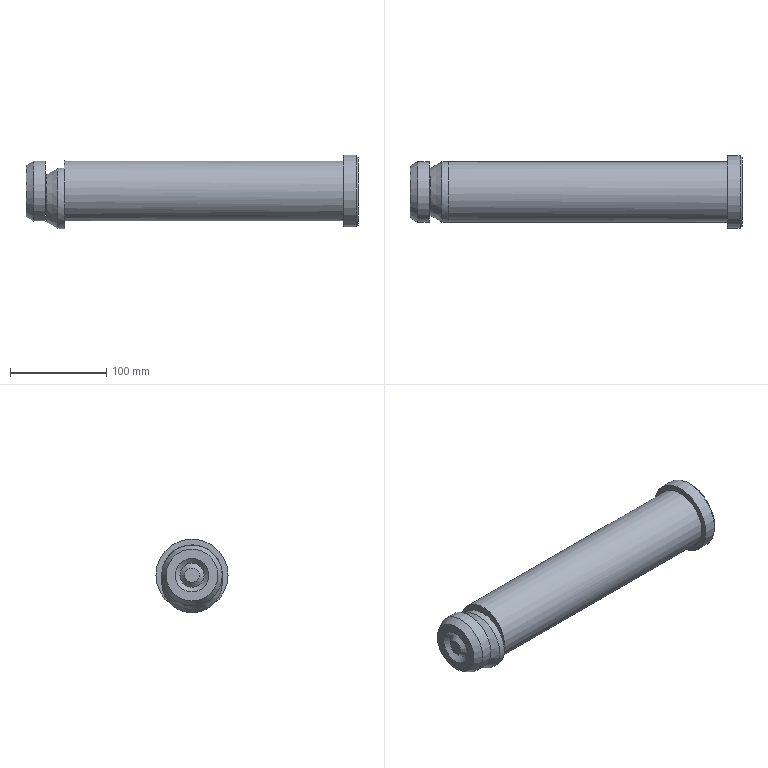Part | NX | features MAIN_BODY 2 | 1 solid | 24 faces | box 345 x 75 x 76.5 mm | volume 1062579 mm3 | plane 10 | cylinder 8 | cone 6 | commonest cylinder face diameters 63 x3 25 x1 25.1 x1 30 x1 44.6 x1 75 x1
STEP:
#1=CARTESIAN_POINT('',(1229.,875.809,-265.597));
#2=VERTEX_POINT('',#1);
#3=CARTESIAN_POINT('',(1229.,884.191,-265.597));
#4=VERTEX_POINT('',#3);
#5=CARTESIAN_POINT('',(1229.,880.,-287.5));
#6=DIRECTION('',(1.,0.,0.));
#7=DIRECTION('',(0.,1.,0.));
#8=AXIS2_PLACEMENT_3D('',#5,#6,#7);
#9=CIRCLE('',#8,22.3);
#10=EDGE_CURVE('',#2,#4,#9,.T.);
#11=ORIENTED_EDGE('',*,*,#10,.F.);
#12=CARTESIAN_POINT('',(1229.,880.,-280.));
#13=DIRECTION('',(1.,0.,0.));
#14=DIRECTION('',(0.,1.,0.));
#15=AXIS2_PLACEMENT_3D('',#12,#13,#14);
#16=CIRCLE('',#15,15.);
#17=EDGE_CURVE('',#2,#4,#16,.T.);
#18=ORIENTED_EDGE('',*,*,#17,.T.);
#19=EDGE_LOOP('',(#11,#18));
#20=FACE_BOUND('',#19,.T.);
#21=CARTESIAN_POINT('',(1229.,880.,-280.));
#22=DIRECTION('',(1.,0.,0.));
#23=DIRECTION('',(0.,1.,0.));
#24=AXIS2_PLACEMENT_3D('',#21,#22,#23);
#25=PLANE('',#24);
#26=ADVANCED_FACE('',(#20),#25,.F.);
#27=CARTESIAN_POINT('',(1209.,895.,-280.));
#28=VERTEX_POINT('',#27);
#29=CARTESIAN_POINT('',(1209.,880.,-280.));
#30=DIRECTION('',(1.,0.,0.));
#31=DIRECTION('',(0.,1.,0.));
#32=AXIS2_PLACEMENT_3D('',#29,#30,#31);
#33=CIRCLE('',#32,15.);
#34=EDGE_CURVE('',#28,#28,#33,.F.);
#35=ORIENTED_EDGE('',*,*,#34,.F.);
#36=EDGE_LOOP('',(#35));
#37=FACE_BOUND('',#36,.T.);
#38=CARTESIAN_POINT('',(1210.,875.809,-265.597));
#39=VERTEX_POINT('',#38);
#40=CARTESIAN_POINT('',(1210.,884.191,-265.597));
#41=VERTEX_POINT('',#40);
#42=CARTESIAN_POINT('',(1210.,880.,-280.));
#43=DIRECTION('',(1.,0.,0.));
#44=DIRECTION('',(0.,1.,0.));
#45=AXIS2_PLACEMENT_3D('',#42,#43,#44);
#46=CIRCLE('',#45,15.);
#47=EDGE_CURVE('',#39,#41,#46,.F.);
#48=ORIENTED_EDGE('',*,*,#47,.T.);
#49=CARTESIAN_POINT('',(1219.6,884.191,-265.597));
#50=DIRECTION('',(1.,0.,0.));
#51=VECTOR('',#50,1000.);
#52=LINE('',#49,#51);
#53=EDGE_CURVE('',#41,#4,#52,.T.);
#54=ORIENTED_EDGE('',*,*,#53,.T.);
#55=ORIENTED_EDGE('',*,*,#17,.F.);
#56=CARTESIAN_POINT('',(1219.6,875.809,-265.597));
#57=DIRECTION('',(1.,0.,0.));
#58=VECTOR('',#57,1000.);
#59=LINE('',#56,#58);
#60=EDGE_CURVE('',#2,#39,#59,.F.);
#61=ORIENTED_EDGE('',*,*,#60,.T.);
#62=EDGE_LOOP('',(#48,#54,#55,#61));
#63=FACE_BOUND('',#62,.T.);
#64=CARTESIAN_POINT('',(1209.,880.,-280.));
#65=DIRECTION('',(1.,0.,0.));
#66=DIRECTION('',(0.,1.,0.));
#67=AXIS2_PLACEMENT_3D('',#64,#65,#66);
#68=CYLINDRICAL_SURFACE('',#67,15.);
#69=ADVANCED_FACE('',(#37,#63),#68,.T.);
#70=CARTESIAN_POINT('',(1208.2,892.55,-280.));
#71=VERTEX_POINT('',#70);
#72=CARTESIAN_POINT('',(1208.2,880.,-280.));
#73=DIRECTION('',(1.,0.,0.));
#74=DIRECTION('',(0.,1.,0.));
#75=AXIS2_PLACEMENT_3D('',#72,#73,#74);
#76=CIRCLE('',#75,12.55);
#77=EDGE_CURVE('',#71,#71,#76,.T.);
#78=ORIENTED_EDGE('',*,*,#77,.T.);
#79=EDGE_LOOP('',(#78));
#80=FACE_BOUND('',#79,.T.);
#81=CARTESIAN_POINT('',(1194.,892.55,-280.));
#82=VERTEX_POINT('',#81);
#83=CARTESIAN_POINT('',(1194.,880.,-280.));
#84=DIRECTION('',(1.,0.,0.));
#85=DIRECTION('',(0.,1.,0.));
#86=AXIS2_PLACEMENT_3D('',#83,#84,#85);
#87=CIRCLE('',#86,12.55);
#88=EDGE_CURVE('',#82,#82,#87,.F.);
#89=ORIENTED_EDGE('',*,*,#88,.T.);
#90=EDGE_LOOP('',(#89));
#91=FACE_BOUND('',#90,.T.);
#92=CARTESIAN_POINT('',(1189.,880.,-280.));
#93=DIRECTION('',(1.,0.,0.));
#94=DIRECTION('',(0.,1.,0.));
#95=AXIS2_PLACEMENT_3D('',#92,#93,#94);
#96=CYLINDRICAL_SURFACE('',#95,12.55);
#97=ADVANCED_FACE('',(#80,#91),#96,.F.);
#98=CARTESIAN_POINT('',(1197.,911.5,-280.));
#99=VERTEX_POINT('',#98);
#100=CARTESIAN_POINT('',(1197.,880.,-280.));
#101=DIRECTION('',(1.,0.,0.));
#102=DIRECTION('',(0.,1.,0.));
#103=AXIS2_PLACEMENT_3D('',#100,#101,#102);
#104=CIRCLE('',#103,31.5);
#105=EDGE_CURVE('',#99,#99,#104,.T.);
#106=ORIENTED_EDGE('',*,*,#105,.T.);
#107=EDGE_LOOP('',(#106));
#108=FACE_BOUND('',#107,.T.);
#109=CARTESIAN_POINT('',(1209.,911.5,-280.));
#110=VERTEX_POINT('',#109);
#111=CARTESIAN_POINT('',(1209.,880.,-280.));
#112=DIRECTION('',(1.,0.,0.));
#113=DIRECTION('',(0.,1.,0.));
#114=AXIS2_PLACEMENT_3D('',#111,#112,#113);
#115=CIRCLE('',#114,31.5);
#116=EDGE_CURVE('',#110,#110,#115,.T.);
#117=ORIENTED_EDGE('',*,*,#116,.F.);
#118=EDGE_LOOP('',(#117));
#119=FACE_BOUND('',#118,.T.);
#120=CARTESIAN_POINT('',(1189.,880.,-280.));
#121=DIRECTION('',(1.,0.,0.));
#122=DIRECTION('',(0.,1.,0.));
#123=AXIS2_PLACEMENT_3D('',#120,#121,#122);
#124=CYLINDRICAL_SURFACE('',#123,31.5);
#125=ADVANCED_FACE('',(#108,#119),#124,.T.);
#126=CARTESIAN_POINT('',(1189.,897.55,-280.));
#127=VERTEX_POINT('',#126);
#128=CARTESIAN_POINT('',(1189.,880.,-280.));
#129=DIRECTION('',(1.,0.,0.));
#130=DIRECTION('',(0.,1.,0.));
#131=AXIS2_PLACEMENT_3D('',#128,#129,#130);
#132=CIRCLE('',#131,17.55);
#133=EDGE_CURVE('',#127,#127,#132,.T.);
#134=ORIENTED_EDGE('',*,*,#133,.T.);
#135=EDGE_LOOP('',(#134));
#136=FACE_BOUND('',#135,.T.);
#137=CARTESIAN_POINT('',(1189.,906.881,-280.));
#138=VERTEX_POINT('',#137);
#139=CARTESIAN_POINT('',(1189.,880.,-280.));
#140=DIRECTION('',(1.,0.,0.));
#141=DIRECTION('',(0.,1.,0.));
#142=AXIS2_PLACEMENT_3D('',#139,#140,#141);
#143=CIRCLE('',#142,26.881);
#144=EDGE_CURVE('',#138,#138,#143,.F.);
#145=ORIENTED_EDGE('',*,*,#144,.T.);
#146=EDGE_LOOP('',(#145));
#147=FACE_BOUND('',#146,.T.);
#148=CARTESIAN_POINT('',(1189.,880.,-280.));
#149=DIRECTION('',(1.,0.,0.));
#150=DIRECTION('',(0.,1.,0.));
#151=AXIS2_PLACEMENT_3D('',#148,#149,#150);
#152=PLANE('',#151);
#153=ADVANCED_FACE('',(#136,#147),#152,.F.);
#154=ORIENTED_EDGE('',*,*,#34,.T.);
#155=EDGE_LOOP('',(#154));
#156=FACE_BOUND('',#155,.T.);
#157=ORIENTED_EDGE('',*,*,#116,.T.);
#158=EDGE_LOOP('',(#157));
#159=FACE_BOUND('',#158,.T.);
#160=CARTESIAN_POINT('',(1209.,880.,-280.));
#161=DIRECTION('',(1.,0.,0.));
#162=DIRECTION('',(0.,1.,0.));
#163=AXIS2_PLACEMENT_3D('',#160,#161,#162);
#164=PLANE('',#163);
#165=ADVANCED_FACE('',(#156,#159),#164,.T.);
#166=ORIENTED_EDGE('',*,*,#144,.F.);
#167=EDGE_LOOP('',(#166));
#168=FACE_BOUND('',#167,.T.);
#169=ORIENTED_EDGE('',*,*,#105,.F.);
#170=EDGE_LOOP('',(#169));
#171=FACE_BOUND('',#170,.T.);
#172=CARTESIAN_POINT('',(1197.,880.,-280.));
#173=DIRECTION('',(1.,0.,0.));
#174=DIRECTION('',(0.,1.,0.));
#175=AXIS2_PLACEMENT_3D('',#172,#173,#174);
#176=CONICAL_SURFACE('',#175,31.5,0.5236);
#177=ADVANCED_FACE('',(#168,#171),#176,.T.);
#178=ORIENTED_EDGE('',*,*,#88,.F.);
#179=EDGE_LOOP('',(#178));
#180=FACE_BOUND('',#179,.T.);
#181=ORIENTED_EDGE('',*,*,#133,.F.);
#182=EDGE_LOOP('',(#181));
#183=FACE_BOUND('',#182,.T.);
#184=CARTESIAN_POINT('',(1189.,880.,-280.));
#185=DIRECTION('',(-1.,0.,0.));
#186=DIRECTION('',(0.,-1.,0.));
#187=AXIS2_PLACEMENT_3D('',#184,#185,#186);
#188=CONICAL_SURFACE('',#187,17.55,0.7854);
#189=ADVANCED_FACE('',(#180,#183),#188,.F.);
#190=CARTESIAN_POINT('',(1209.,893.35,-280.));
#191=VERTEX_POINT('',#190);
#192=CARTESIAN_POINT('',(1209.,880.,-280.));
#193=DIRECTION('',(1.,0.,0.));
#194=DIRECTION('',(0.,1.,0.));
#195=AXIS2_PLACEMENT_3D('',#192,#193,#194);
#196=CIRCLE('',#195,13.35);
#197=EDGE_CURVE('',#191,#191,#196,.F.);
#198=ORIENTED_EDGE('',*,*,#197,.F.);
#199=EDGE_LOOP('',(#198));
#200=FACE_BOUND('',#199,.T.);
#201=ORIENTED_EDGE('',*,*,#77,.F.);
#202=EDGE_LOOP('',(#201));
#203=FACE_BOUND('',#202,.T.);
#204=CARTESIAN_POINT('',(1208.2,880.,-280.));
#205=DIRECTION('',(1.,0.,0.));
#206=DIRECTION('',(0.,1.,0.));
#207=AXIS2_PLACEMENT_3D('',#204,#205,#206);
#208=CONICAL_SURFACE('',#207,12.55,0.7854);
#209=ADVANCED_FACE('',(#200,#203),#208,.F.);
#210=CARTESIAN_POINT('',(1189.,887.5,-280.));
#211=VERTEX_POINT('',#210);
#212=CARTESIAN_POINT('',(1189.,880.,-280.));
#213=DIRECTION('',(1.,0.,0.));
#214=DIRECTION('',(0.,1.,0.));
#215=AXIS2_PLACEMENT_3D('',#212,#213,#214);
#216=CIRCLE('',#215,7.5);
#217=EDGE_CURVE('',#211,#211,#216,.F.);
#218=ORIENTED_EDGE('',*,*,#217,.T.);
#219=EDGE_LOOP('',(#218));
#220=FACE_BOUND('',#219,.T.);
#221=CARTESIAN_POINT('',(1189.,880.,-280.));
#222=DIRECTION('',(1.,0.,0.));
#223=DIRECTION('',(0.,1.,0.));
#224=AXIS2_PLACEMENT_3D('',#221,#222,#223);
#225=PLANE('',#224);
#226=ADVANCED_FACE('',(#220),#225,.F.);
#227=ORIENTED_EDGE('',*,*,#217,.F.);
#228=EDGE_LOOP('',(#227));
#229=FACE_BOUND('',#228,.T.);
#230=CARTESIAN_POINT('',(1194.,892.5,-280.));
#231=VERTEX_POINT('',#230);
#232=CARTESIAN_POINT('',(1194.,880.,-280.));
#233=DIRECTION('',(1.,0.,0.));
#234=DIRECTION('',(0.,1.,0.));
#235=AXIS2_PLACEMENT_3D('',#232,#233,#234);
#236=CIRCLE('',#235,12.5);
#237=EDGE_CURVE('',#231,#231,#236,.T.);
#238=ORIENTED_EDGE('',*,*,#237,.F.);
#239=EDGE_LOOP('',(#238));
#240=FACE_BOUND('',#239,.T.);
#241=CARTESIAN_POINT('',(1194.,880.,-280.));
#242=DIRECTION('',(1.,0.,0.));
#243=DIRECTION('',(0.,1.,0.));
#244=AXIS2_PLACEMENT_3D('',#241,#242,#243);
#245=CONICAL_SURFACE('',#244,12.5,0.7854);
#246=ADVANCED_FACE('',(#229,#240),#245,.T.);
#247=ORIENTED_EDGE('',*,*,#237,.T.);
#248=EDGE_LOOP('',(#247));
#249=FACE_BOUND('',#248,.T.);
#250=CARTESIAN_POINT('',(1209.,892.5,-280.));
#251=VERTEX_POINT('',#250);
#252=CARTESIAN_POINT('',(1209.,880.,-280.));
#253=DIRECTION('',(1.,0.,0.));
#254=DIRECTION('',(0.,1.,0.));
#255=AXIS2_PLACEMENT_3D('',#252,#253,#254);
#256=CIRCLE('',#255,12.5);
#257=EDGE_CURVE('',#251,#251,#256,.T.);
#258=ORIENTED_EDGE('',*,*,#257,.F.);
#259=EDGE_LOOP('',(#258));
#260=FACE_BOUND('',#259,.T.);
#261=CARTESIAN_POINT('',(1189.,880.,-280.));
#262=DIRECTION('',(1.,0.,0.));
#263=DIRECTION('',(0.,1.,0.));
#264=AXIS2_PLACEMENT_3D('',#261,#262,#263);
#265=CYLINDRICAL_SURFACE('',#264,12.5);
#266=ADVANCED_FACE('',(#249,#260),#265,.T.);
#267=ORIENTED_EDGE('',*,*,#197,.T.);
#268=EDGE_LOOP('',(#267));
#269=FACE_BOUND('',#268,.T.);
#270=ORIENTED_EDGE('',*,*,#257,.T.);
#271=EDGE_LOOP('',(#270));
#272=FACE_BOUND('',#271,.T.);
#273=CARTESIAN_POINT('',(1209.,880.,-280.));
#274=DIRECTION('',(1.,0.,0.));
#275=DIRECTION('',(0.,1.,0.));
#276=AXIS2_PLACEMENT_3D('',#273,#274,#275);
#277=PLANE('',#276);
#278=ADVANCED_FACE('',(#269,#272),#277,.F.);
#279=ORIENTED_EDGE('',*,*,#53,.F.);
#280=CARTESIAN_POINT('',(1210.,880.,-287.5));
#281=DIRECTION('',(1.,0.,0.));
#282=DIRECTION('',(0.,1.,0.));
#283=AXIS2_PLACEMENT_3D('',#280,#281,#282);
#284=CIRCLE('',#283,22.3);
#285=EDGE_CURVE('',#39,#41,#284,.T.);
#286=ORIENTED_EDGE('',*,*,#285,.F.);
#287=ORIENTED_EDGE('',*,*,#60,.F.);
#288=ORIENTED_EDGE('',*,*,#10,.T.);
#289=EDGE_LOOP('',(#279,#286,#287,#288));
#290=FACE_BOUND('',#289,.T.);
#291=CARTESIAN_POINT('',(1210.,880.,-287.5));
#292=DIRECTION('',(1.,0.,0.));
#293=DIRECTION('',(0.,1.,0.));
#294=AXIS2_PLACEMENT_3D('',#291,#292,#293);
#295=CYLINDRICAL_SURFACE('',#294,22.3);
#296=ADVANCED_FACE('',(#290),#295,.F.);
#297=CARTESIAN_POINT('',(1222.124,911.5,-287.5));
#298=VERTEX_POINT('',#297);
#299=CARTESIAN_POINT('',(1222.124,880.,-287.5));
#300=DIRECTION('',(1.,0.,0.));
#301=DIRECTION('',(0.,1.,0.));
#302=AXIS2_PLACEMENT_3D('',#299,#300,#301);
#303=CIRCLE('',#302,31.5);
#304=EDGE_CURVE('',#298,#298,#303,.T.);
#305=ORIENTED_EDGE('',*,*,#304,.T.);
#306=EDGE_LOOP('',(#305));
#307=FACE_BOUND('',#306,.T.);
#308=CARTESIAN_POINT('',(1229.,911.276,-283.75));
#309=VERTEX_POINT('',#308);
#310=CARTESIAN_POINT('',(1229.,848.724,-283.75));
#311=VERTEX_POINT('',#310);
#312=CARTESIAN_POINT('',(1229.,880.,-287.5));
#313=DIRECTION('',(1.,0.,0.));
#314=DIRECTION('',(0.,1.,0.));
#315=AXIS2_PLACEMENT_3D('',#312,#313,#314);
#316=CIRCLE('',#315,31.5);
#317=EDGE_CURVE('',#309,#311,#316,.T.);
#318=ORIENTED_EDGE('',*,*,#317,.F.);
#319=CARTESIAN_POINT('',(1229.2,911.276,-283.75));
#320=VERTEX_POINT('',#319);
#321=CARTESIAN_POINT('',(1229.1,911.276,-283.75));
#322=DIRECTION('',(1.,0.,0.));
#323=VECTOR('',#322,1000.);
#324=LINE('',#321,#323);
#325=EDGE_CURVE('',#309,#320,#324,.T.);
#326=ORIENTED_EDGE('',*,*,#325,.T.);
#327=CARTESIAN_POINT('',(1229.2,848.724,-283.75));
#328=VERTEX_POINT('',#327);
#329=CARTESIAN_POINT('',(1229.2,880.,-287.5));
#330=DIRECTION('',(1.,0.,0.));
#331=DIRECTION('',(0.,1.,0.));
#332=AXIS2_PLACEMENT_3D('',#329,#330,#331);
#333=CIRCLE('',#332,31.5);
#334=EDGE_CURVE('',#328,#320,#333,.T.);
#335=ORIENTED_EDGE('',*,*,#334,.F.);
#336=CARTESIAN_POINT('',(1229.1,848.724,-283.75));
#337=DIRECTION('',(1.,0.,0.));
#338=VECTOR('',#337,1000.);
#339=LINE('',#336,#338);
#340=EDGE_CURVE('',#328,#311,#339,.F.);
#341=ORIENTED_EDGE('',*,*,#340,.T.);
#342=EDGE_LOOP('',(#318,#326,#335,#341));
#343=FACE_BOUND('',#342,.T.);
#344=CARTESIAN_POINT('',(1210.,880.,-287.5));
#345=DIRECTION('',(1.,0.,0.));
#346=DIRECTION('',(0.,1.,0.));
#347=AXIS2_PLACEMENT_3D('',#344,#345,#346);
#348=CYLINDRICAL_SURFACE('',#347,31.5);
#349=ADVANCED_FACE('',(#307,#343),#348,.T.);
#350=ORIENTED_EDGE('',*,*,#47,.F.);
#351=ORIENTED_EDGE('',*,*,#285,.T.);
#352=EDGE_LOOP('',(#350,#351));
#353=FACE_BOUND('',#352,.T.);
#354=CARTESIAN_POINT('',(1210.,904.5,-287.5));
#355=VERTEX_POINT('',#354);
#356=CARTESIAN_POINT('',(1210.,880.,-287.5));
#357=DIRECTION('',(1.,0.,0.));
#358=DIRECTION('',(0.,1.,0.));
#359=AXIS2_PLACEMENT_3D('',#356,#357,#358);
#360=CIRCLE('',#359,24.5);
#361=EDGE_CURVE('',#355,#355,#360,.F.);
#362=ORIENTED_EDGE('',*,*,#361,.T.);
#363=EDGE_LOOP('',(#362));
#364=FACE_BOUND('',#363,.T.);
#365=CARTESIAN_POINT('',(1210.,880.,-287.5));
#366=DIRECTION('',(1.,0.,0.));
#367=DIRECTION('',(0.,1.,0.));
#368=AXIS2_PLACEMENT_3D('',#365,#366,#367);
#369=PLANE('',#368);
#370=ADVANCED_FACE('',(#353,#364),#369,.F.);
#371=ORIENTED_EDGE('',*,*,#334,.T.);
#372=CARTESIAN_POINT('',(1229.2,880.,-280.));
#373=DIRECTION('',(1.,0.,0.));
#374=DIRECTION('',(0.,1.,0.));
#375=AXIS2_PLACEMENT_3D('',#372,#373,#374);
#376=CIRCLE('',#375,31.5);
#377=EDGE_CURVE('',#320,#328,#376,.F.);
#378=ORIENTED_EDGE('',*,*,#377,.T.);
#379=EDGE_LOOP('',(#371,#378));
#380=FACE_BOUND('',#379,.T.);
#381=CARTESIAN_POINT('',(1229.2,880.,-287.5));
#382=DIRECTION('',(1.,0.,0.));
#383=DIRECTION('',(0.,1.,0.));
#384=AXIS2_PLACEMENT_3D('',#381,#382,#383);
#385=PLANE('',#384);
#386=ADVANCED_FACE('',(#380),#385,.T.);
#387=ORIENTED_EDGE('',*,*,#361,.F.);
#388=EDGE_LOOP('',(#387));
#389=FACE_BOUND('',#388,.T.);
#390=ORIENTED_EDGE('',*,*,#304,.F.);
#391=EDGE_LOOP('',(#390));
#392=FACE_BOUND('',#391,.T.);
#393=CARTESIAN_POINT('',(1222.124,880.,-287.5));
#394=DIRECTION('',(1.,0.,0.));
#395=DIRECTION('',(0.,1.,0.));
#396=AXIS2_PLACEMENT_3D('',#393,#394,#395);
#397=CONICAL_SURFACE('',#396,31.5,0.5236);
#398=ADVANCED_FACE('',(#389,#392),#397,.T.);
#399=CARTESIAN_POINT('',(1534.,915.5,-280.));
#400=VERTEX_POINT('',#399);
#401=CARTESIAN_POINT('',(1534.,880.,-280.));
#402=DIRECTION('',(1.,0.,0.));
#403=DIRECTION('',(0.,1.,0.));
#404=AXIS2_PLACEMENT_3D('',#401,#402,#403);
#405=CIRCLE('',#404,35.5);
#406=EDGE_CURVE('',#400,#400,#405,.T.);
#407=ORIENTED_EDGE('',*,*,#406,.T.);
#408=EDGE_LOOP('',(#407));
#409=FACE_BOUND('',#408,.T.);
#410=CARTESIAN_POINT('',(1534.,880.,-280.));
#411=DIRECTION('',(1.,0.,0.));
#412=DIRECTION('',(0.,1.,0.));
#413=AXIS2_PLACEMENT_3D('',#410,#411,#412);
#414=PLANE('',#413);
#415=ADVANCED_FACE('',(#409),#414,.T.);
#416=CARTESIAN_POINT('',(1532.,917.5,-280.));
#417=VERTEX_POINT('',#416);
#418=CARTESIAN_POINT('',(1532.,880.,-280.));
#419=DIRECTION('',(1.,0.,0.));
#420=DIRECTION('',(0.,1.,0.));
#421=AXIS2_PLACEMENT_3D('',#418,#419,#420);
#422=CIRCLE('',#421,37.5);
#423=EDGE_CURVE('',#417,#417,#422,.F.);
#424=ORIENTED_EDGE('',*,*,#423,.F.);
#425=EDGE_LOOP('',(#424));
#426=FACE_BOUND('',#425,.T.);
#427=ORIENTED_EDGE('',*,*,#406,.F.);
#428=EDGE_LOOP('',(#427));
#429=FACE_BOUND('',#428,.T.);
#430=CARTESIAN_POINT('',(1534.,880.,-280.));
#431=DIRECTION('',(-1.,0.,0.));
#432=DIRECTION('',(0.,-1.,0.));
#433=AXIS2_PLACEMENT_3D('',#430,#431,#432);
#434=CONICAL_SURFACE('',#433,35.5,0.7854);
#435=ADVANCED_FACE('',(#426,#429),#434,.T.);
#436=ORIENTED_EDGE('',*,*,#423,.T.);
#437=EDGE_LOOP('',(#436));
#438=FACE_BOUND('',#437,.T.);
#439=CARTESIAN_POINT('',(1519.,917.5,-280.));
#440=VERTEX_POINT('',#439);
#441=CARTESIAN_POINT('',(1519.,880.,-280.));
#442=DIRECTION('',(1.,0.,0.));
#443=DIRECTION('',(0.,1.,0.));
#444=AXIS2_PLACEMENT_3D('',#441,#442,#443);
#445=CIRCLE('',#444,37.5);
#446=EDGE_CURVE('',#440,#440,#445,.T.);
#447=ORIENTED_EDGE('',*,*,#446,.T.);
#448=EDGE_LOOP('',(#447));
#449=FACE_BOUND('',#448,.T.);
#450=CARTESIAN_POINT('',(1519.,880.,-280.));
#451=DIRECTION('',(1.,0.,0.));
#452=DIRECTION('',(0.,1.,0.));
#453=AXIS2_PLACEMENT_3D('',#450,#451,#452);
#454=CYLINDRICAL_SURFACE('',#453,37.5);
#455=ADVANCED_FACE('',(#438,#449),#454,.T.);
#456=CARTESIAN_POINT('',(1519.,911.5,-280.));
#457=VERTEX_POINT('',#456);
#458=CARTESIAN_POINT('',(1519.,880.,-280.));
#459=DIRECTION('',(1.,0.,0.));
#460=DIRECTION('',(0.,1.,0.));
#461=AXIS2_PLACEMENT_3D('',#458,#459,#460);
#462=CIRCLE('',#461,31.5);
#463=EDGE_CURVE('',#457,#457,#462,.T.);
#464=ORIENTED_EDGE('',*,*,#463,.T.);
#465=EDGE_LOOP('',(#464));
#466=FACE_BOUND('',#465,.T.);
#467=ORIENTED_EDGE('',*,*,#446,.F.);
#468=EDGE_LOOP('',(#467));
#469=FACE_BOUND('',#468,.T.);
#470=CARTESIAN_POINT('',(1519.,880.,-280.));
#471=DIRECTION('',(1.,0.,0.));
#472=DIRECTION('',(0.,1.,0.));
#473=AXIS2_PLACEMENT_3D('',#470,#471,#472);
#474=PLANE('',#473);
#475=ADVANCED_FACE('',(#466,#469),#474,.F.);
#476=CARTESIAN_POINT('',(1229.,880.,-280.));
#477=DIRECTION('',(1.,0.,0.));
#478=DIRECTION('',(0.,1.,0.));
#479=AXIS2_PLACEMENT_3D('',#476,#477,#478);
#480=CIRCLE('',#479,31.5);
#481=EDGE_CURVE('',#309,#311,#480,.T.);
#482=ORIENTED_EDGE('',*,*,#481,.F.);
#483=ORIENTED_EDGE('',*,*,#317,.T.);
#484=EDGE_LOOP('',(#482,#483));
#485=FACE_BOUND('',#484,.T.);
#486=CARTESIAN_POINT('',(1229.,880.,-280.));
#487=DIRECTION('',(1.,0.,0.));
#488=DIRECTION('',(0.,1.,0.));
#489=AXIS2_PLACEMENT_3D('',#486,#487,#488);
#490=PLANE('',#489);
#491=ADVANCED_FACE('',(#485),#490,.F.);
#492=ORIENTED_EDGE('',*,*,#325,.F.);
#493=ORIENTED_EDGE('',*,*,#481,.T.);
#494=ORIENTED_EDGE('',*,*,#340,.F.);
#495=ORIENTED_EDGE('',*,*,#377,.F.);
#496=EDGE_LOOP('',(#492,#493,#494,#495));
#497=FACE_BOUND('',#496,.T.);
#498=ORIENTED_EDGE('',*,*,#463,.F.);
#499=EDGE_LOOP('',(#498));
#500=FACE_BOUND('',#499,.T.);
#501=CARTESIAN_POINT('',(1229.,880.,-280.));
#502=DIRECTION('',(1.,0.,0.));
#503=DIRECTION('',(0.,1.,0.));
#504=AXIS2_PLACEMENT_3D('',#501,#502,#503);
#505=CYLINDRICAL_SURFACE('',#504,31.5);
#506=ADVANCED_FACE('',(#497,#500),#505,.T.);
#507=CLOSED_SHELL('',(#26,#69,#97,#125,#153,#165,#177,#189,#209,#226,#246,#266,#278,#296,#349,#370,#386,#398,#415,#435,#455,#475,#491,#506));
#508=MANIFOLD_SOLID_BREP('',#507);
#509=(LENGTH_UNIT()NAMED_UNIT(*)SI_UNIT(.MILLI.,.METRE.));
#510=UNCERTAINTY_MEASURE_WITH_UNIT(LENGTH_MEASURE(0.00001),#509,'','');
#511=(NAMED_UNIT(*)PLANE_ANGLE_UNIT()SI_UNIT($,.RADIAN.));
#512=(NAMED_UNIT(*)SI_UNIT($,.STERADIAN.)SOLID_ANGLE_UNIT());
#513=(GEOMETRIC_REPRESENTATION_CONTEXT(3)GLOBAL_UNCERTAINTY_ASSIGNED_CONTEXT((#510))GLOBAL_UNIT_ASSIGNED_CONTEXT((#509,#511,#512))REPRESENTATION_CONTEXT('',''));
#514=ADVANCED_BREP_SHAPE_REPRESENTATION('',(#508),#513);